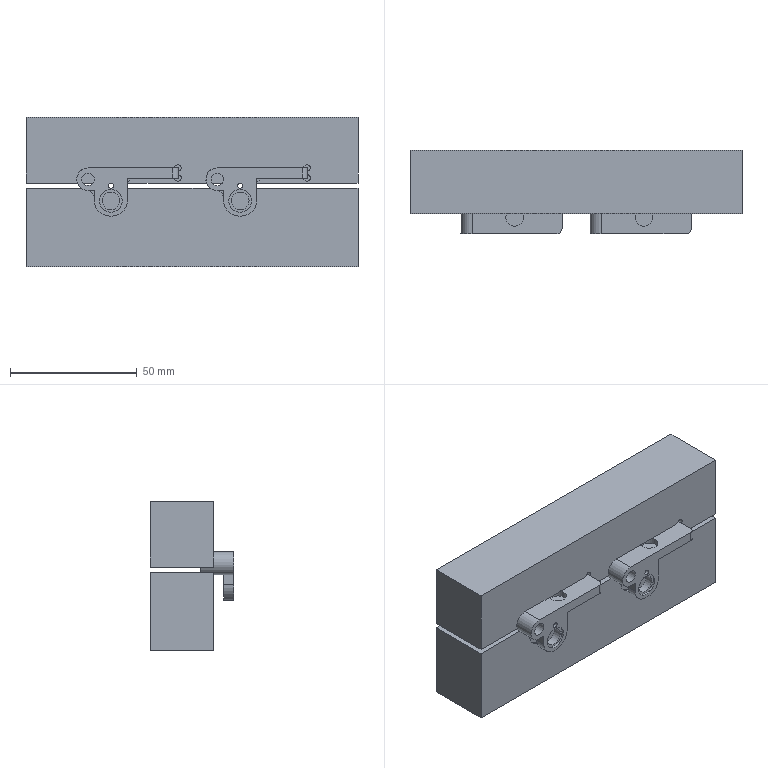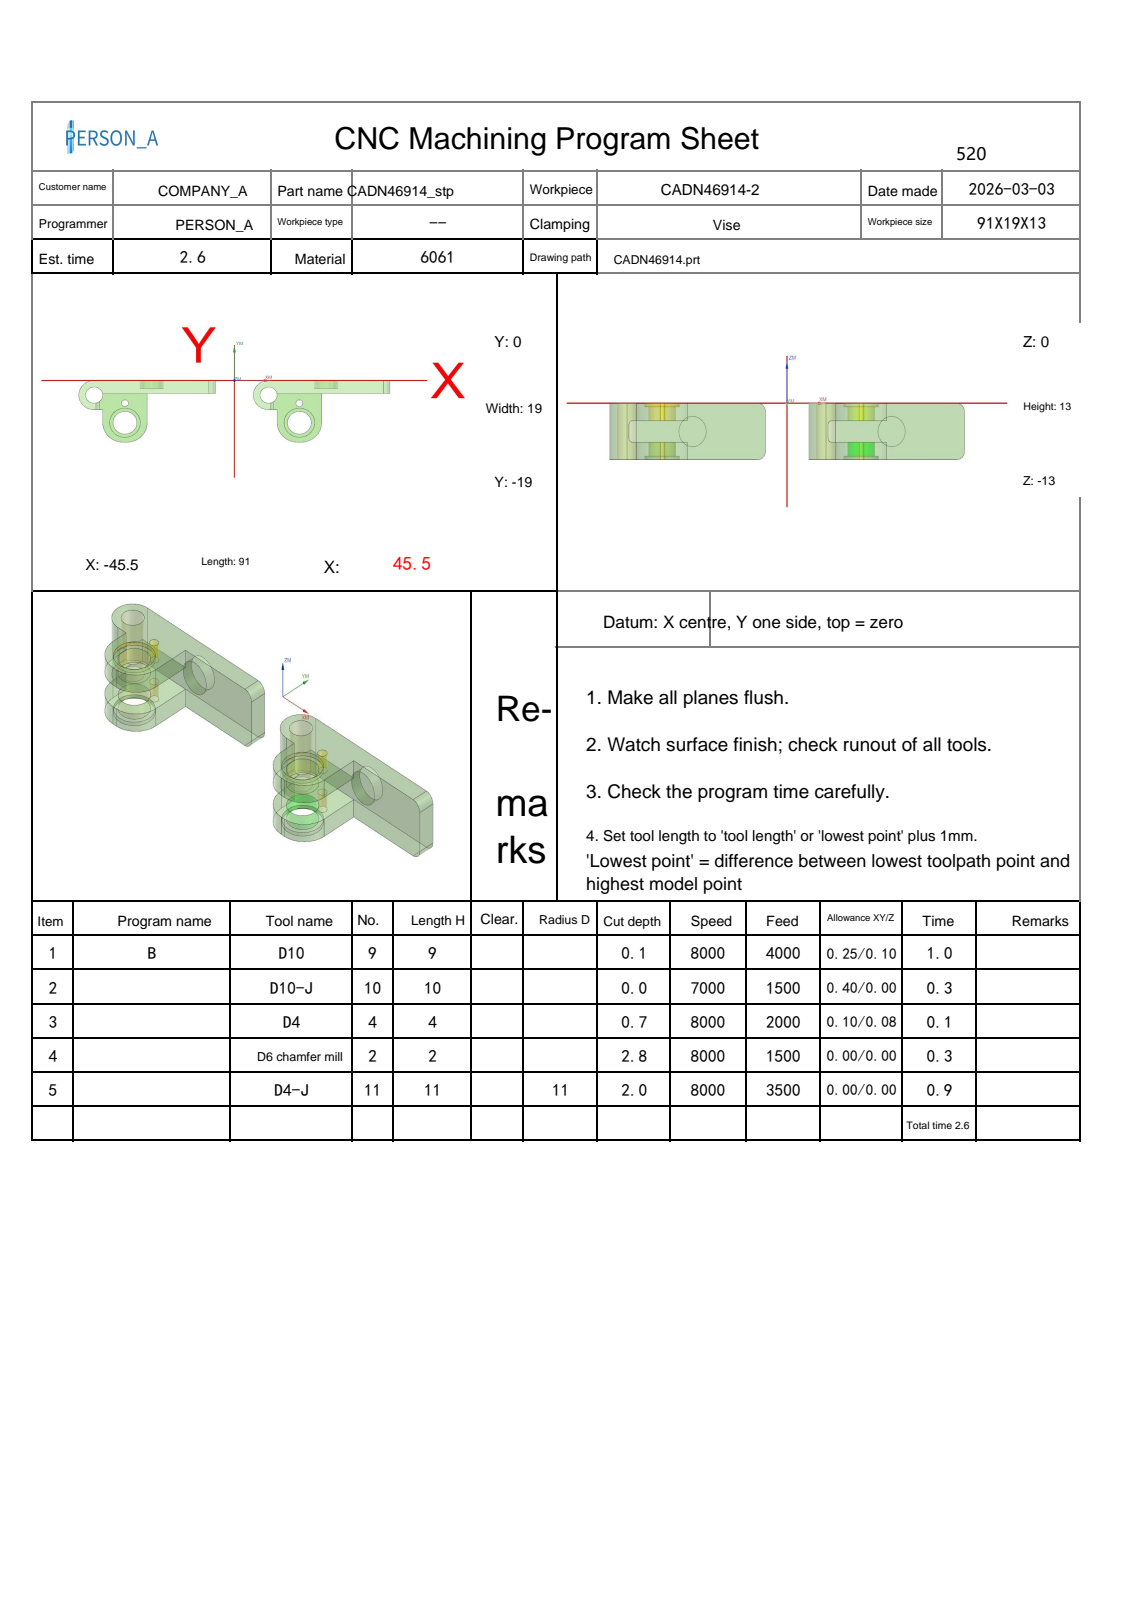NC program | NX | posted by the shop | part box 131 x 33 x 59 mm
Lines 1 to 823 of 3834:
%
O0001
(Machine time: 3.66 MIN)
(===Total Tool:5===)
(T9=D10     D=10.  R=0.   D-  H09 Z=0.1   )
(T10=D10-J  D=10.  R=0.   D-  H10 Z=0.    )
(T4=D4      D=4.   R=0.   D-  H04 Z=-0.74 )
(T2=D6 chamfer mill   D=6.   R=0.   D-  H02 Z=-2.8  )
(T11=D4-J   D=4.   R=0.   D11 H11 Z=-2.   )
G80 G90 G17 G49 G40
G91 G28 Z0
M01
N1 T09 M06
(D10  D=10. R=0. H=09 ce=0.25 di=0.10)
G00 G90 G54 X-30.909 Y-31.155 M03 S8000
G43 H09 Z50.
M08
Z2.1
G01 X-30.927 Y-31.057 Z1.476 F4000.
X-30.945 Y-30.959 Z1.228
X-30.963 Y-30.86 Z1.046
X-30.981 Y-30.762 Z.9
X-30.999 Y-30.664 Z.777
X-31.017 Y-30.565 Z.672
X-31.035 Y-30.467 Z.58
X-31.053 Y-30.369 Z.5
X-31.071 Y-30.27 Z.43
X-31.089 Y-30.172 Z.368
X-31.107 Y-30.073 Z.314
X-31.125 Y-29.975 Z.267
X-31.143 Y-29.877 Z.227
X-31.161 Y-29.778 Z.192
X-31.179 Y-29.68 Z.164
X-31.197 Y-29.582 Z.14
X-31.215 Y-29.483 Z.123
X-31.233 Y-29.385 Z.11
X-31.251 Y-29.287 Z.103
X-31.269 Y-29.188 Z.1
X-31.683 Y-26.928
G03 X-31.974 Y-26.557 I-.503 J-.096
X-35.369 Y-26.025 I-3.395 J-10.561
G01 X-35.378
G03 X-45.758 Y-25.878 I-10.38 J-366.896
G01 X-46.534 Y-25.879
G02 X-53.31 Y-20.868 I.094 J7.214
X-54.282 Y-14.911 I19.145 J6.183
X-54.408 Y-6.217 I301.605 J8.693
X-54.356 Y-.655 I301.73 J0.0
X-49.462 Y5.772 I7.159 J-.375
X-43.751 Y6.768 I6.091 J-18.05
X-34.458 Y6.913 I9.294 J-298.23
X-31.633 Y6.9 I0.0 J-298.375
G01 X46.484 Y6.88
G02 X53.339 Y1.805 I-.055 J-7.242
X54.29 Y-4.217 I-19.603 J-6.183
X54.408 Y-12.723 I-307.222 J-8.506
X54.356 Y-18.343 I-307.34 J0.0
X49.36 Y-24.821 I-7.196 J.384
X43.402 Y-25.789 I-6.162 J19.115
X34.109 Y-25.908 I-9.293 J361.438
X31.643 Y-25.9 I0.0 J361.557
G01 X-29.852 Y-25.879
G03 X-42.962 Y-25.287 I-13.11 J-144.776
X-44.565 Y-25.296 I0.0 J-145.369
G01 X-44.745 Y-25.298
G02 X-52.141 Y-20.418 I0.0 J8.044
X-53.578 Y-14.067 I16.695 J7.116
X-53.806 Y-6.34 I130.755 J7.728
X-53.732 Y-1.954 I130.983 J0.0
X-49.068 Y4.566 I7.909 J-.73
X-42.798 Y6.062 I7.116 J-15.936
X-34.185 Y6.311 I8.613 J-148.4
X-32.124 Y6.297 I0.0 J-148.65
G01 X44.983 Y6.275
G02 X52.084 Y1.54 I-.183 J-7.965
X53.568 Y-4.79 I-16.14 J-7.122
X53.804 Y-12.719 I-132.822 J-7.929
X53.734 Y-17.023 I-133.059 J0.0
X49.191 Y-23.511 I-7.874 J.68
X42.877 Y-25.057 I-7.147 J15.517
X34.204 Y-25.313 I-8.672 J147.08
X32.082 Y-25.298 I0.0 J147.336
G01 X-28.352 Y-25.282
G03 X-38.121 Y-24.785 I-31.414 J-521.043
G01 X-38.186
G02 X-44.289 Y-24.627 I0.0 J117.678
X-51.299 Y-19.517 I1.01 J8.748
X-52.928 Y-12.784 I17.191 J7.725
X-53.177 Y-6.467 I80.034 J6.317
X-53.117 Y-3.372 I80.283 J0.0
X-47.928 Y3.838 I8.761 J-.833
X-41.431 Y5.418 I7.602 J-17.121
X-32.17 Y5.714 I9.261 J-144.374
X-29.918 Y5.697 I0.0 J-144.671
G01 X43.382 Y5.679
G02 X51.328 Y.458 I-.112 J-8.827
X52.908 Y-5.979 I-16.969 J-7.578
X53.182 Y-12.373 I-74.292 J-6.393
X53.106 Y-15.75 I-74.567 J0.0
X47.926 Y-22.845 I-8.741 J.944
X41.43 Y-24.42 I-7.592 J17.134
X32.972 Y-24.703 I-8.458 J126.042
X31.477 Y-24.694 I0.0 J126.326
G01 X-27.152 Y-24.683
G02 X-36.777 Y-24.24 I33.127 J823.91
X-43. Y-24.029 I.831 J116.329
X-50.686 Y-18.315 I1.087 J9.489
X-52.31 Y-11.399 I18.803 J8.063
X-52.53 Y-6.998 I43.818 J4.401
X-52.457 Y-4.448 I44.039 J0.0
X-46.886 Y3.143 I9.381 J-1.045
X-39.921 Y4.81 I8.097 J-18.451
X-30.714 Y5.108 I9.207 J-142.294
X-28.828 Y5.095 I0.0 J-142.592
G01 X41.952 Y5.076
G02 X50.709 Y-.738 I-.046 J-9.57
X52.299 Y-7.478 I-18.669 J-7.963
X52.531 Y-11.968 I-43.227 J-4.49
X52.451 Y-14.608 I-43.459 J0.0
X46.996 Y-22.095 I-9.342 J1.077
X40.102 Y-23.795 I-8.086 J17.958
X30.379 Y-24.115 I-9.723 J147.719
X28.049 Y-24.096 I0.0 J148.038
G01 X-26.291 Y-24.081
G02 X-37.007 Y-23.643 I27.352 J800.964
G01 X-37.131
G02 X-42.246 Y-23.376 I0.0 J49.068
X-50.019 Y-17.334 I1.555 J10.022
X-51.702 Y-10.063 I19.966 J8.451
X-51.854 Y-7.567 I20.434 J2.496
X-51.65 Y-4.679 I20.586 J0.0
X-45.928 Y2.456 I9.731 J-1.942
X-38.665 Y4.194 I8.463 J-19.315
X-28.877 Y4.51 I9.788 J-151.501
X-26.732 Y4.495 I0.0 J-151.816
G01 X40.568 Y4.475
X40.658
G02 X47.996 Y1.362 I0.0 J-10.204
X51.155 Y-5.148 I-10.168 J-8.956
X51.835 Y-11.488 I-29.221 J-6.339
X51.759 Y-13.618 I-29.901 J0.0
X45.932 Y-21.458 I-9.817 J1.212
X38.911 Y-23.173 I-8.357 J18.981
X29.938 Y-23.498 I-8.973 J123.647
X28.6 Y-23.491 I0.0 J123.972
G01 X-25.92 Y-23.473
G02 X-40.239 Y-22.9 I21.622 J719.624
X-49.458 Y-16.195 I.747 J10.718
X-51.085 Y-7.96 I20.031 J8.234
X-51.019 Y-6.267 I21.658 J0.0
X-45.11 Y1.731 I10.096 J-1.277
X-37.928 Y3.539 I8.647 J-19.177
X-28.301 Y3.903 I9.627 J-127.259
X-26.598 Y3.892 I0.0 J-127.623
G01 X39.022 Y3.881
G02 X39.247 Y3.883 I.225 J-11.752
X45.366 Y2.165 I0.0 J-11.754
X50.022 Y-4.311 I-6.737 J-9.755
X51.084 Y-11.056 I-20.892 J-6.745
X51.021 Y-12.719 I-21.954 J0.0
X45.275 Y-20.652 I-10.048 J1.231
X38.046 Y-22.529 I-8.707 J18.678
X28.597 Y-22.9 I-9.45 J120.055
X27.077 Y-22.89 I0.0 J120.426
G01 X-25.223 Y-22.873
G02 X-39.236 Y-22.313 I7.28 J358.195
X-48.822 Y-15.279 I.825 J11.172
X-50.266 Y-8.423 I15.546 J6.856
X-50.198 Y-6.902 I16.991 J0.0
X-44.529 Y.903 I10.151 J-1.413
X-37.155 Y2.892 I8.966 J-18.572
X-27.335 Y3.301 I9.821 J-117.746
X-25.707 Y3.289 I0.0 J-118.155
G01 X37.753 Y3.28
G02 X38.004 Y3.282 I.251 J-12.992
X43.943 Y1.846 I0.0 J-12.994
X49.105 Y-4.45 I-5.899 J-10.101
X50.265 Y-10.554 I-15.478 J-6.104
X50.182 Y-12.222 I-16.638 J0.0
X44.532 Y-19.905 I-10.138 J1.536
X37.159 Y-21.893 I-8.963 J18.577
X27.305 Y-22.301 I-9.853 J118.59
X25.65 Y-22.29 I0.0 J118.999
G01 X-24.67 Y-22.271
G02 X-38.168 Y-21.741 I3.868 J270.513
X-48.177 Y-14.427 I.787 J11.583
X-49.375 Y-8.924 I12.044 J5.503
X-49.241 Y-7.045 I13.242 J0.0
X-43.664 Y.227 I10.109 J-1.978
X-36.24 Y2.264 I9.118 J-18.688
X-26.123 Y2.701 I10.117 J-116.94
X-24.433 Y2.689 I0.0 J-117.377
G01 X36.747 Y2.673
X36.934 Y2.675
G02 X43.059 Y1.223 I0.0 J-13.64
X48.506 Y-5.446 I-5.983 J-10.447
X49.377 Y-10.013 I-11.536 J-4.567
X49.109 Y-12.576 I-12.407 J0.0
X43.475 Y-19.329 I-10.081 J2.686
X36.082 Y-21.283 I-9.067 J19.34
X25.918 Y-21.702 I-10.164 J122.867
X24.154 Y-21.69 I0.0 J123.286
G01 X-23.826 Y-21.675
G02 X-37.211 Y-21.162 I1.64 J217.921
X-45.171 Y-17.364 I.855 J12.032
X-48.402 Y-9.096 I8.964 J8.268
X-48.381 Y-8.392 I12.195 J0.0
X-43.357 Y-.765 I9.905 J-1.056
X-36.081 Y1.544 I9.282 J-16.632
X-26.268 Y2.083 I9.813 J-89.064
X-25.241 Y2.077 I0.0 J-89.603
G01 X35.279 Y2.081
G02 X35.607 Y2.084 I.328 J-15.86
X41.383 Y.995 I0.0 J-15.864
X48.024 Y-6.942 I-4.94 J-10.879
X48.409 Y-9.66 I-9.393 J-2.718
X43.694 Y-18.026 I-9.778 J0.0
X36.472 Y-20.489 I-9.34 J15.566
X27.077 Y-21.066 I-9.395 J76.115
X26.536 Y-21.064 I0.0 J76.693
G01 X17.176 Y-21.097
X-23.544 Y-21.071
G02 X-36.132 Y-20.601 I1.135 J199.048
X-43.611 Y-17.532 I.864 J12.756
X-47.348 Y-9.404 I7.131 J8.201
X-42.876 Y-1.705 I9.541 J-.394
X-35.81 Y.821 I9.344 J-14.99
X-26.106 Y1.465 I9.704 J-72.839
X-25.459 Y1.462 I0.0 J-73.482
G01 X-15.979 Y1.496
X34.461 Y1.473
G02 X34.697 Y1.475 I.236 J-15.947
X40.783 Y.268 I0.0 J-15.949
X47.325 Y-9.029 I-4.475 J-10.099
X47.328 Y-9.271 I-9.442 J-.242
X42.987 Y-17.218 I-9.445 J0.0
X35.819 Y-19.821 I-9.405 J14.734
X26.383 Y-20.456 I-9.436 J69.748
X26.008 Y-20.455 I0.0 J70.383
G01 X16.048 Y-20.496
X-23.292 Y-20.468
G02 X-35.221 Y-20.023 I.513 J174.128
X-42.506 Y-17.208 I.931 J13.245
X-46.178 Y-9.87 I5.933 J7.556
X-42.09 Y-2.491 I9.163 J-.254
X-35.232 Y.135 I9.298 J-14.014
X-25.806 Y.842 I9.427 J-62.498
G01 X-25.607
X-15.047 Y.896
X33.232 Y.876
G02 X33.542 Y.879 I.31 J-17.647
X39.53 Y-.168 I0.0 J-17.65
X45.906 Y-7.131 I-3.657 J-9.75
X46.127 Y-9.086 I-8.527 J-1.955
X42.809 Y-15.946 I-8.748 J0.0
X35.964 Y-18.994 I-9.449 J12.005
X26.713 Y-19.819 I-9.326 J52.329
X16.426 Y-19.898 I-10.287 J668.029
X14.774 Y-19.896 I0.0 J668.108
G01 X-22.466 Y-19.871
G02 X-34.216 Y-19.457 I.048 J168.294
X-41.208 Y-17.005 I.926 J13.835
X-44.89 Y-10.064 I4.85 J7.02
X-40.98 Y-3.097 I8.834 J-.378
X-34.196 Y-.477 I9.199 J-13.725
X-24.75 Y.239 I9.446 J-61.973
G01 X-24.573
X-12.573 Y.296
X32.227 Y.274
G02 X32.549 Y.277 I.323 J-18.504
X38.649 Y-.757 I0.0 J-18.507
X44.255 Y-5.922 I-3.271 J-9.175
X44.821 Y-8.894 I-7.527 J-2.971
X42.302 Y-14.76 I-8.092 J0.0
X36.074 Y-18.109 I-9.259 J9.752
X27.515 Y-19.158 I-9.158 J39.295
X15.299 Y-19.307 I-12.217 J499.276
X11.977 Y-19.296 I0.0 J499.426
G01 X-22.443 Y-19.266
X-22.465
G02 X-33.294 Y-18.883 I0.0 J153.275
X-39.808 Y-16.816 I.949 J14.287
X-43.459 Y-10.329 I3.935 J6.486
X-43.417 Y-9.528 I7.587 J0.0
X-39.254 Y-3.337 I8.705 J-1.359
X-32.437 Y-.971 I9. J-14.928
X-22.843 Y-.344 I9.593 J-73.025
X-22.385 Y-.345 I0.0 J-73.653
G01 X-11.045 Y-.305
X31.175 Y-.325
G02 X31.531 Y-.322 I.356 J-19.654
X37.67 Y-1.305 I0.0 J-19.658
X42.687 Y-5.548 I-2.755 J-8.347
X43.377 Y-8.695 I-6.839 J-3.147
X41.368 Y-13.815 I-7.528 J0.0
X35.303 Y-17.401 I-9.12 J8.503
X27.176 Y-18.522 I-8.951 J34.867
X14.657 Y-18.713 I-12.52 J409.322
X10.858 Y-18.696 I0.0 J409.513
G01 X-21.641 Y-18.67
X-22.127 Y-18.671
G02 X-32.492 Y-18.297 I0.0 J143.913
X-38.429 Y-16.545 I.978 J14.249
X-41.895 Y-10.558 I3.438 J5.987
X-40.605 Y-6.54 I6.904 J0.0
X-35.043 Y-2.508 I8.873 J-6.388
X-27.262 Y-1.149 I8.845 J-27.671
X-16.643 Y-.9 I10.619 J-226.324
X-14.667 Y-.908 I0.0 J-226.573
G01 X30.073 Y-.924
G02 X30.483 Y-.92 I.409 J-21.216
X36.47 Y-1.782 I0.0 J-21.22
X41.107 Y-5.525 I-2.149 J-7.406
X41.765 Y-8.5 I-6.39 J-2.975
X40.047 Y-13.112 I-7.048 J0.0
X34.236 Y-16.744 I-8.84 J7.676
X26.42 Y-17.9 I-8.741 J32.117
X14.543 Y-18.111 I-11.877 J334.585
X11.303 Y-18.095 I0.0 J334.796
G01 X-20.837 Y-18.073
G02 X-21.609 Y-18.075 I-.772 J140.422
X-31.628 Y-17.717 I0.0 J140.424
X-36.866 Y-16.304 I.898 J13.74
X-40.139 Y-10.762 I3.054 J5.542
X-39.284 Y-7.586 I6.328 J0.0
X-34.238 Y-3.332 I8.473 J-4.931
X-26.923 Y-1.815 I8.557 J-22.87
X-16.193 Y-1.497 I10.731 J-180.624
X-14.03 Y-1.51 I0.0 J-180.943
G01 X29.03 Y-1.523
G02 X29.477 Y-1.518 I.447 J-22.469
X35.205 Y-2.261 I0.0 J-22.474
X39.746 Y-6.64 I-1.597 J-6.201
X39.933 Y-8.242 I-6.788 J-1.601
X37.81 Y-13.252 I-6.974 J0.0
X31.887 Y-16.415 I-8.532 J8.851
X23.497 Y-17.374 I-8.793 J39.753
X11.633 Y-17.501 I-11.865 J552.436
X8.978 Y-17.495 I0.0 J552.563
G01 X-20.281 Y-17.474
G02 X-21.122 Y-17.476 I-.84 J137.747
X-30.713 Y-17.142 I0.0 J137.749
X-35.113 Y-16.053 I.676 J12.165
X-38.142 Y-10.973 I2.747 J5.08
X-37.639 Y-8.616 I5.775 J0.0
X-32.92 Y-4.051 I8.097 J-3.65
X-25.934 Y-2.449 I8.26 J-19.982
X-16.106 Y-2.108 I9.828 J-141.461
X-14.662 Y-2.115 I0.0 J-141.802
G01 X28.518 Y-2.132
G02 X28.842 Y-2.129 I.324 J-20.333
X33.923 Y-2.774 I0.0 J-20.335
X37.875 Y-8.127 I-1.647 J-5.352
X37.481 Y-10.19 I-5.6 J0.0
X32.987 Y-14.843 I-7.943 J3.176
X26.202 Y-16.517 I-8.149 J18.435
X16.154 Y-16.897 I-10.048 J132.809
X14.452 Y-16.886 I0.0 J133.188
G01 X-20.328 Y-16.87
G02 X-21.277 Y-16.874 I-.949 J114.103
X-30.159 Y-16.527 I0.0 J114.107
X-33.666 Y-15.425 I.324 J7.159
X-35.804 Y-11.14 I3.225 J4.285
X-35.392 Y-9.08 I5.363 J0.0
X-30.97 Y-4.622 I7.696 J-3.213
X-24.408 Y-3.055 I7.83 J-18.262
X-14.836 Y-2.707 I9.572 J-131.589
X-13.377 Y-2.715 I0.0 J-131.937
G01 X27.223 Y-2.725
G02 X27.649 Y-2.721 I.426 J-21.726
X31.757 Y-3.113 I0.0 J-21.731
X35.386 Y-7.913 I-1.362 J-4.8
X35.252 Y-9.061 I-4.99 J0.0
X31.372 Y-14.023 I-7.364 J1.76
X25.19 Y-15.84 I-7.687 J14.735
X16.228 Y-16.279 I-8.962 J91.153
X15.305 Y-16.275 I0.0 J91.593
G01 X-19.775 Y-16.271
G02 X-20.771 Y-16.275 I-.996 J110.02
X-29.067 Y-15.962 I0.0 J110.025
X-32.969 Y-11.448 I.66 J4.514
X-32.933 Y-10.876 I4.562 J0.0
X-29.591 Y-5.774 I6.889 J-.867
X-23.591 Y-3.791 I7.471 J-12.542
X-14.918 Y-3.321 I8.674 J-79.779
X-13.949 Y-3.327 I0.0 J-80.249
G01 X26.591 Y-3.331
G02 X27.007 Y-3.323 I.416 J-10.767
X29.331 Y-3.576 I0.0 J-10.775
X32.272 Y-7.719 I-1.447 J-4.143
X32.241 Y-8.238 I-4.388 J0.0
X29.006 Y-13.256 I-6.734 J.79
X23.005 Y-15.236 I-7.368 J12.246
X14.37 Y-15.685 I-8.635 J82.781
X13.241 Y-15.677 I0.0 J83.23
G01 X-18.959 Y-15.674
X-19.265
G02 X-26.215 Y-15.506 I0.0 J143.369
X-29.274 Y-11.956 I.778 J3.764
X-29.285 Y-11.597 I6.076 J.359
X-26.806 Y-6.695 I6.086 J0.0
X-21.122 Y-4.438 I7.151 J-9.722
X-13.235 Y-3.928 I7.887 J-60.726
X-12.445 Y-3.933 I0.0 J-61.236
G01 X25.035 Y-3.926
G02 X27.803 Y-6.204 I-.437 J-3.351
X28.111 Y-7.97 I-4.914 J-1.766
X26.338 Y-11.89 I-5.222 J0.0
X21.045 Y-14.432 I-7.004 J7.802
X13.752 Y-15.048 I-7.293 J42.86
X13.4 Y-15.047 I0.0 J43.476
G01 X4.34 Y-15.093
X-19.82 Y-15.063
G02 X-20.421 Y-15.078 I-.601 J12.185
X-22.033 Y-14.971 I0.0 J12.2
X-24.422 Y-11.89 I1.476 J3.611
X-24.48 Y-11.1 I5.345 J.79
X-21.163 Y-6.116 I5.403 J0.0
X-15.172 Y-4.736 I6.737 J-15.564
X-6.507 Y-4.497 I8.666 J-156.443
X-4.497 Y-4.51 I0.0 J-156.682
G01 X19.957 Y-4.528
G02 X22.561 Y-8.37 I-1.532 J-3.842
G01 X22.56 Y-8.484
G02 X17.927 Y-13.799 I-5.412 J.04
X10.995 Y-14.439 I-6.932 J37.223
G01 X10.767 Y-14.438
X1.767 Y-14.492
X-14.072 Y-14.514
G03 X-15.978 Y-14.733 I4.452 J-47.149
X-16.346 Y-15.032 I.099 J-.497
X-16.115 Y-15.677 Z.138 I.488 J-.189
G01 X-15.141 Y-16.432 Z.2
X-13.347 Y-17.823
X-13.282 Y-17.866
X-13.21 Y-17.898
X-13.135 Y-17.919
X-13.057 Y-17.927
X-12.979 Y-17.924
X-12.903 Y-17.908
X-12.829 Y-17.881
X-12.647 Y-17.796
X-12.574 Y-17.754
X-12.508 Y-17.7
X-12.453 Y-17.635
X-12.409 Y-17.563
X-12.379 Y-17.484
X-12.362 Y-17.401
X-12.359 Y-17.316
X-12.371 Y-17.232
X-12.396 Y-17.152
X-12.435 Y-17.076
X-12.486 Y-17.009
X-12.548 Y-16.951
X-14.249 Y-15.603
X-15.283 Y-14.775 Z.133
G02 X-15.335 Y-14.169 Z.1 I.372 J.336
X-14.911 Y-13.938 I.424 J-.274
G01 X-14.873 Y-13.94
G03 X-.918 Y-14.038 I13.955 J997.184
X6.715 Y-14.008 I0.0 J997.281
X10.404 Y-14.322 I3.689 J21.545
X11.076 Y-14.312 I0.0 J21.858
G01 X11.176 Z.103
X11.276 Y-14.313 Z.11
X11.376 Z.123
X11.476 Y-14.314 Z.14
X11.576 Z.164
X11.676 Y-14.315 Z.192
X11.776 Z.227
X11.876 Y-14.316 Z.267
X11.976 Z.314
X12.076 Y-14.317 Z.368
X12.176 Y-14.318 Z.43
X12.276 Z.5
X12.376 Y-14.319 Z.58
X12.476 Z.672
X12.576 Y-14.32 Z.777
X12.676 Z.9
X12.776 Y-14.321 Z1.046
X12.876 Z1.228
X12.976 Y-14.322 Z1.476
X13.076 Z2.1
G00 Z50.
G91 G28 Z0.0
M05
M09
G91 G28 Z0.0
M01
N2 T10 M06
(D10-J  D=10. R=0. H=10 ce=0.40 di=0.00)
G00 G90 G54 X-50.806 Y1.508 M03 S7000
G43 H10 Z11.8
M08
Z1.5
G01 Z0.0 F1500.
G03 X-49.123 Y.589 I1.682 J1.081
G01 X-49.02 Y.592
X-3.447 Y2.951
X-3.4 Y2.952
G02 X-2.5 Y2.052 I0.0 J-.9
G01 Y-.176
G02 X-3.448 Y-1.174 I-1. J0.0
G01 X-49.552 Y-3.561
G03 X-50.5 Y-4.559 I.052 J-.999
G01 Y-4.566
G03 X-50.186 Y-6.923 I9.5 J.066
X-49.219 Y-7.668 I.967 J.255
G01 X-49.167 Y-7.666
X-3.446 Y-5.299
X-3.4 Y-5.298
G02 X-2.5 Y-6.198 I0.0 J-.9
G01 Y-8.07
G02 X-3.427 Y-9.067 I-1. J0.0
G01 X-20.49 Y-10.307
X-20.51 Y-10.308
X-46.295 Y-11.643
G03 X-46.674 Y-12.043 I.021 J-.399
X-46.553 Y-12.329 I.4 J0.0
G01 X-43.5 Y-15.303
G03 X-42.802 Y-15.586 I.698 J.716
G01 X-42.75 Y-15.585
X-20.594 Y-14.438
G03 X-18.698 Y-12.441 I-.103 J1.997
G01 X-18.7 Y-12.337
X-18.5
Z1.5
G00 Z4.
X.194 Y1.508
Z1.5
G01 Z0.0
G03 X1.877 Y.589 I1.682 J1.081
G01 X1.98 Y.592
X47.553 Y2.951
X47.6 Y2.953
G02 X48.5 Y2.053 I0.0 J-.9
G01 Y-.176
G02 X47.552 Y-1.174 I-1. J0.0
G01 X1.448 Y-3.561
G03 X.5 Y-4.56 I.052 J-.999
G01 Y-4.566
G03 X.814 Y-6.923 I9.5 J.066
X1.781 Y-7.668 I.967 J.255
G01 X1.833 Y-7.666
X47.554 Y-5.299
X47.6 Y-5.298
G02 X48.5 Y-6.198 I0.0 J-.9
G01 Y-8.07
G02 X47.573 Y-9.067 I-1. J0.0
G01 X30.51 Y-10.307
X30.49 Y-10.308
X4.705 Y-11.643
G03 X4.326 Y-12.043 I.021 J-.399
X4.447 Y-12.329 I.4 J0.0
G01 X7.501 Y-15.303
G03 X8.198 Y-15.586 I.698 J.716
G01 X8.25 Y-15.585
X30.406 Y-14.438
G03 X32.302 Y-12.441 I-.103 J1.997
G01 X32.3 Y-12.337
X32.5
Z1.5
G00 Z11.8
G91 G28 Z0.0
M05
M09
G91 G28 Z0.0
M01
N3 T04 M06
(D4  D=4. R=0. H=04 ce=0.10 di=0.08)
G00 G90 G54 X-32.098 Y-15.4 M03 S8000
G43 H04 Z50.
M08
Z1.
G01 X-31.619 Z.975 F2000.
X-30.676 Y-15.038 Z.922
X-29.962 Y-14.324 Z.869
X-29.6 Y-13.381 Z.816
Y-12.619 Z.776
X-29.962 Y-11.676 Z.723
X-30.676 Y-10.962 Z.67
X-31.619 Y-10.6 Z.617
X-32.381 Z.577
X-33.324 Y-10.962 Z.525
X-34.038 Y-11.676 Z.472
X-34.4 Y-12.619 Z.419
Y-13.381 Z.379
X-34.038 Y-14.324 Z.326
X-33.324 Y-15.038 Z.273
X-32.381 Y-15.4 Z.22
X-32. Z.2
G03 X-29.6 Y-13. Z.141 I0.0 J2.4
X-32. Y-10.6 Z.083 I-2.4 J0.0
X-34.4 Y-13. Z.024 I0.0 J-2.4
X-32. Y-15.4 Z-.035 I2.4 J0.0
X-29.6 Y-13. Z-.094 I0.0 J2.4
X-32. Y-10.6 Z-.153 I-2.4 J0.0
X-34.4 Y-13. Z-.211 I0.0 J-2.4
X-32. Y-15.4 Z-.27 I2.4 J0.0
X-29.6 Y-13. Z-.329 I0.0 J2.4
X-32. Y-10.6 Z-.388 I-2.4 J0.0
X-34.4 Y-13. Z-.446 I0.0 J-2.4
X-32. Y-15.4 Z-.505 I2.4 J0.0
X-29.6 Y-13. Z-.564 I0.0 J2.4
X-32. Y-10.6 Z-.623 I-2.4 J0.0
X-34.4 Y-13. Z-.681 I0.0 J-2.4
X-32. Y-15.4 Z-.74 I2.4 J0.0
X-29.6 Y-13. I0.0 J2.4
X-32. Y-10.6 I-2.4 J0.0
X-34.4 Y-13. I0.0 J-2.4
X-32. Y-15.4 I2.4 J0.0
X-31.602 Y-15.367 I0.0 J2.4
G01 Z.06
G00 Z50.
X18.907 Y-15.4
Z1.
G01 X19.381 Z.975
X20.324 Y-15.038 Z.922
X21.038 Y-14.324 Z.869
X21.4 Y-13.381 Z.816
Y-12.619 Z.776
X21.059 Y-11.709 Z.726
X20.388 Y-11.005 Z.675
X19.703 Y-10.674 Z.635
X19.381 Y-10.6 Z.617
X18.619 Z.577
X17.676 Y-10.962 Z.525
X16.962 Y-11.676 Z.472
X16.6 Y-12.619 Z.419
Y-13.381 Z.379
X16.962 Y-14.324 Z.326
X17.676 Y-15.038 Z.273
X18.619 Y-15.4 Z.22
X19. Z.2
G03 X21.4 Y-13. Z.141 I0.0 J2.4
X20.045 Y-10.84 Z.099 I-2.4 J0.0
X19. Y-10.6 Z.083 I-1.045 J-2.16
X16.6 Y-13. Z.024 I0.0 J-2.4
X19. Y-15.4 Z-.035 I2.4 J0.0
X21.4 Y-13. Z-.094 I0.0 J2.4
X20.045 Y-10.84 Z-.136 I-2.4 J0.0
X19. Y-10.6 Z-.153 I-1.045 J-2.16
X16.6 Y-13. Z-.211 I0.0 J-2.4
X19. Y-15.4 Z-.27 I2.4 J0.0
X21.4 Y-13. Z-.329 I0.0 J2.4
X20.045 Y-10.84 Z-.371 I-2.4 J0.0
X19. Y-10.6 Z-.388 I-1.045 J-2.16
X16.6 Y-13. Z-.446 I0.0 J-2.4
X19. Y-15.4 Z-.505 I2.4 J0.0
X21.4 Y-13. Z-.564 I0.0 J2.4
X20.045 Y-10.84 Z-.606 I-2.4 J0.0
X19. Y-10.6 Z-.623 I-1.045 J-2.16
X16.6 Y-13. Z-.681 I0.0 J-2.4
X19. Y-15.4 Z-.74 I2.4 J0.0
X21.4 Y-13. I0.0 J2.4
X19. Y-10.6 I-2.4 J0.0
X16.6 Y-13. I0.0 J-2.4
X19. Y-15.4 I2.4 J0.0
X19.398 Y-15.367 I0.0 J2.4
G01 Z.06
G00 Z50.
G91 G28 Z0.0
M05
M09
G91 G28 Z0.0
M01
N4 T02 M06
(D6 chamfer mill  D=6. R=0. H=02 ce=0.00 di=0.08)
G00 G90 G54 X10. Y-4.5 M03 S8000
G43 H02 Z50.
M08
G98 G81 X10. Y-4.5 Z-2.8 R3. F1000.
X-41.
G80
G00 Z50.
G00 G90 X19. Y-7. M03 S8000
Z50.
G98 G81 X19. Y-7. Z-1.475 R3. F500.
X-32.
G80
G00 Z50.
G00 G90 X-7.114 Y-4.727 M03 S6500
Z50.
Z.637
G01 Z-.7 F1500.
G03 X-7.4 Y-4.527 I-1.286 J-1.532
G01 X-7.446 Y-4.497
X-7.5 Y-4.5
X-25.
Y-13.
G02 X-31.5 Y-19.5 I-6.5 J0.0
G01 X-32.5
G02 X-39. Y-13. I0.0 J6.5
G01 Y-9.5
X-41.
G02 X-46. Y-4.5 I0.0 J5.
X-41. Y.5 I5. J0.0
G01 X-7.5
X-7.446 Y.497
X-7.4 Y.527
G03 X-7.114 Y.727 I-1. J1.732
G01 Z.637
G00 Z10.
X-31.6 Y-9.201
Z.721
G01 Z-.7
G03 X-31.898 Y-9.02 I-1.183 J-1.613
G01 X-31.946 Y-8.994
X-32. Y-9.
G03 X-36. Y-13. I0.0 J-4.
X-32. Y-17. I4. J0.0
X-28. Y-13. I0.0 J4.
X-32. Y-9. I-4. J0.0
G01 X-32.054 Y-8.994
X-32.102 Y-9.02
G03 X-32.4 Y-9.201 I.885 J-1.794
G01 Z.721
G00 Z3.05
X-40.596 Y-2.692
Z.759
G01 Z-.7
G03 X-40.898 Y-2.518 I-1.147 J-1.638
G01 X-40.946 Y-2.492
X-41. Y-2.5
G03 X-43. Y-4.5 I0.0 J-2.
X-41. Y-6.5 I2. J0.0
X-39. Y-4.5 I0.0 J2.
X-40.653 Y-2.53 I-2. J0.0
G01 X-41. Y-2.5
X-41.054 Y-2.492
X-41.102 Y-2.518
G03 X-41.404 Y-2.692 I.845 J-1.813
G01 Z.759
G00 Z10.
X43.886 Y-4.727
Z.637
G01 Z-.7
G03 X43.6 Y-4.527 I-1.286 J-1.532
G01 X43.554 Y-4.497
X43.5 Y-4.5
X26.
Y-13.
G02 X19.5 Y-19.5 I-6.5 J0.0
G01 X18.5
G02 X12. Y-13. I0.0 J6.5
G01 Y-9.5
X10.
G02 X5. Y-4.5 I0.0 J5.
X10. Y.5 I5. J0.0
G01 X43.5
X43.554 Y.497
X43.6 Y.527
G03 X43.886 Y.727 I-1. J1.732
G01 Z.637
G00 Z10.
X19.4 Y-9.201
Z.721
G01 Z-.7
G03 X19.102 Y-9.02 I-1.183 J-1.613
G01 X19.054 Y-8.994
X19. Y-9.
G03 X15. Y-13. I0.0 J-4.
X19. Y-17. I4. J0.0
X23. Y-13. I0.0 J4.
X19. Y-9. I-4. J0.0
G01 X18.946 Y-8.994
X18.898 Y-9.02
G03 X18.6 Y-9.201 I.885 J-1.794
G01 Z.721
G00 Z3.05
X10.404 Y-2.692
Z.759
G01 Z-.7
G03 X10.102 Y-2.518 I-1.147 J-1.638
G01 X10.054 Y-2.492
X10. Y-2.5
G03 X8. Y-4.5 I0.0 J-2.
X10. Y-6.5 I2. J0.0
X12. Y-4.5 I0.0 J2.
X10.347 Y-2.53 I-2. J0.0
G01 X10. Y-2.5
X9.946 Y-2.492
X9.898 Y-2.518
G03 X9.596 Y-2.692 I.845 J-1.813
G01 Z.759
G00 Z10.
X19.401 Y-10.197
Z-.06
G01 Z-1.5
G03 X19.102 Y-10.019 I-1.167 J-1.624
G01 X19.054 Y-9.993
X19. Y-10.
G03 X16. Y-13. I0.0 J-3.
X19. Y-16. I3. J0.0
X22. Y-13. I0.0 J3.
X19. Y-10. I-3. J0.0
G01 X18.946 Y-9.993
X18.898 Y-10.019
G03 X18.599 Y-10.197 I.868 J-1.802
G01 Z-.06
G00 Z10.
X-31.599
Z-.06
G01 Z-1.5
G03 X-31.898 Y-10.019 I-1.167 J-1.624
G01 X-31.946 Y-9.993
X-32. Y-10.
G03 X-35. Y-13. I0.0 J-3.
X-32. Y-16. I3. J0.0
X-29. Y-13. I0.0 J3.
X-32. Y-10. I-3. J0.0
G01 X-32.054 Y-9.993
X-32.102 Y-10.019
G03 X-32.401 Y-10.197 I.868 J-1.802
G01 Z-.06
G00 Z50.
G91 G28 Z0.0
M05
M09
G91 G28 Z0.0
M01